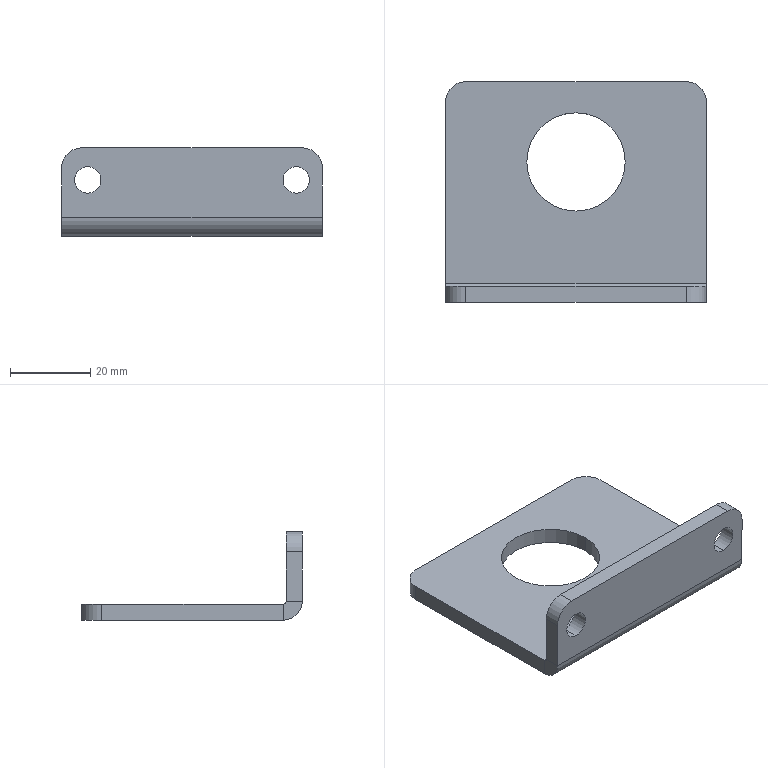Part | SolidWorks | features EdgeFlange 1, Fillet 1, FlatPattern 1, HoleWzd 1, ICE 1, SMBaseFlange 1, SheetMetal 1 | 1 solid | 24 faces | box 65 x 55 x 22 mm | volume 16429 mm3 | cylinder 12 | plane 12 | commonest cylinder face diameters 6.6 x4 10 x4 24.5 x2 1.473 x1 9.473 x1
STEP:
#1=CARTESIAN_POINT('',(-26.,-27.5,6.7));
#2=VERTEX_POINT('',#1);
#3=CARTESIAN_POINT('',(-26.,-27.5,13.3));
#4=VERTEX_POINT('',#3);
#5=CARTESIAN_POINT('',(-26.,-27.5,10.));
#6=DIRECTION('',(0.,1.,0.));
#7=DIRECTION('',(0.,0.,1.));
#8=AXIS2_PLACEMENT_3D('',#5,#6,#7);
#9=CIRCLE('',#8,3.3);
#10=EDGE_CURVE('',#2,#4,#9,.T.);
#11=ORIENTED_EDGE('',*,*,#10,.F.);
#12=CARTESIAN_POINT('',(-26.,-23.5,6.7));
#13=VERTEX_POINT('',#12);
#14=CARTESIAN_POINT('',(-26.,-23.5,6.7));
#15=DIRECTION('',(0.,1.,0.));
#16=VECTOR('',#15,1000.);
#17=LINE('',#14,#16);
#18=EDGE_CURVE('',#2,#13,#17,.T.);
#19=ORIENTED_EDGE('',*,*,#18,.T.);
#20=CARTESIAN_POINT('',(-26.,-23.5,13.3));
#21=VERTEX_POINT('',#20);
#22=CARTESIAN_POINT('',(-26.,-23.5,10.));
#23=DIRECTION('',(0.,1.,0.));
#24=DIRECTION('',(0.,0.,1.));
#25=AXIS2_PLACEMENT_3D('',#22,#23,#24);
#26=CIRCLE('',#25,3.3);
#27=EDGE_CURVE('',#13,#21,#26,.T.);
#28=ORIENTED_EDGE('',*,*,#27,.T.);
#29=CARTESIAN_POINT('',(-26.,-23.5,13.3));
#30=DIRECTION('',(0.,1.,0.));
#31=VECTOR('',#30,1000.);
#32=LINE('',#29,#31);
#33=EDGE_CURVE('',#4,#21,#32,.T.);
#34=ORIENTED_EDGE('',*,*,#33,.F.);
#35=EDGE_LOOP('',(#11,#19,#28,#34));
#36=FACE_OUTER_BOUND('',#35,.T.);
#37=CARTESIAN_POINT('',(-26.,-23.5,10.));
#38=DIRECTION('',(0.,1.,0.));
#39=DIRECTION('',(0.,0.,1.));
#40=AXIS2_PLACEMENT_3D('',#37,#38,#39);
#41=CYLINDRICAL_SURFACE('',#40,3.3);
#42=ADVANCED_FACE('',(#36),#41,.F.);
#43=CARTESIAN_POINT('',(26.,-27.5,6.7));
#44=VERTEX_POINT('',#43);
#45=CARTESIAN_POINT('',(26.,-27.5,13.3));
#46=VERTEX_POINT('',#45);
#47=CARTESIAN_POINT('',(26.,-27.5,10.));
#48=DIRECTION('',(0.,1.,0.));
#49=DIRECTION('',(0.,0.,1.));
#50=AXIS2_PLACEMENT_3D('',#47,#48,#49);
#51=CIRCLE('',#50,3.3);
#52=EDGE_CURVE('',#44,#46,#51,.T.);
#53=ORIENTED_EDGE('',*,*,#52,.F.);
#54=CARTESIAN_POINT('',(26.,-23.5,6.7));
#55=VERTEX_POINT('',#54);
#56=CARTESIAN_POINT('',(26.,-23.5,6.7));
#57=DIRECTION('',(0.,1.,0.));
#58=VECTOR('',#57,1000.);
#59=LINE('',#56,#58);
#60=EDGE_CURVE('',#44,#55,#59,.T.);
#61=ORIENTED_EDGE('',*,*,#60,.T.);
#62=CARTESIAN_POINT('',(26.,-23.5,13.3));
#63=VERTEX_POINT('',#62);
#64=CARTESIAN_POINT('',(26.,-23.5,10.));
#65=DIRECTION('',(0.,1.,0.));
#66=DIRECTION('',(0.,0.,1.));
#67=AXIS2_PLACEMENT_3D('',#64,#65,#66);
#68=CIRCLE('',#67,3.3);
#69=EDGE_CURVE('',#55,#63,#68,.T.);
#70=ORIENTED_EDGE('',*,*,#69,.T.);
#71=CARTESIAN_POINT('',(26.,-23.5,13.3));
#72=DIRECTION('',(0.,1.,0.));
#73=VECTOR('',#72,1000.);
#74=LINE('',#71,#73);
#75=EDGE_CURVE('',#46,#63,#74,.T.);
#76=ORIENTED_EDGE('',*,*,#75,.F.);
#77=EDGE_LOOP('',(#53,#61,#70,#76));
#78=FACE_OUTER_BOUND('',#77,.T.);
#79=CARTESIAN_POINT('',(26.,-23.5,10.));
#80=DIRECTION('',(0.,1.,0.));
#81=DIRECTION('',(0.,0.,1.));
#82=AXIS2_PLACEMENT_3D('',#79,#80,#81);
#83=CYLINDRICAL_SURFACE('',#82,3.3);
#84=ADVANCED_FACE('',(#78),#83,.F.);
#85=CARTESIAN_POINT('',(12.25,7.5,0.));
#86=VERTEX_POINT('',#85);
#87=CARTESIAN_POINT('',(-12.25,7.5,0.));
#88=VERTEX_POINT('',#87);
#89=CARTESIAN_POINT('',(0.,7.5,0.));
#90=DIRECTION('',(0.,0.,-1.));
#91=DIRECTION('',(-1.,0.,0.));
#92=AXIS2_PLACEMENT_3D('',#89,#90,#91);
#93=CIRCLE('',#92,12.25);
#94=EDGE_CURVE('',#86,#88,#93,.T.);
#95=ORIENTED_EDGE('',*,*,#94,.F.);
#96=CARTESIAN_POINT('',(12.25,7.5,-4.));
#97=VERTEX_POINT('',#96);
#98=CARTESIAN_POINT('',(12.25,7.5,18.));
#99=DIRECTION('',(0.,0.,-1.));
#100=VECTOR('',#99,1000.);
#101=LINE('',#98,#100);
#102=EDGE_CURVE('',#86,#97,#101,.T.);
#103=ORIENTED_EDGE('',*,*,#102,.T.);
#104=CARTESIAN_POINT('',(-12.25,7.5,-4.));
#105=VERTEX_POINT('',#104);
#106=CARTESIAN_POINT('',(0.,7.5,-4.));
#107=DIRECTION('',(0.,0.,-1.));
#108=DIRECTION('',(-1.,0.,0.));
#109=AXIS2_PLACEMENT_3D('',#106,#107,#108);
#110=CIRCLE('',#109,12.25);
#111=EDGE_CURVE('',#97,#105,#110,.T.);
#112=ORIENTED_EDGE('',*,*,#111,.T.);
#113=CARTESIAN_POINT('',(-12.25,7.5,18.));
#114=DIRECTION('',(0.,0.,-1.));
#115=VECTOR('',#114,1000.);
#116=LINE('',#113,#115);
#117=EDGE_CURVE('',#88,#105,#116,.T.);
#118=ORIENTED_EDGE('',*,*,#117,.F.);
#119=EDGE_LOOP('',(#95,#103,#112,#118));
#120=FACE_OUTER_BOUND('',#119,.T.);
#121=CARTESIAN_POINT('',(0.,7.5,18.));
#122=DIRECTION('',(0.,0.,-1.));
#123=DIRECTION('',(-1.,0.,0.));
#124=AXIS2_PLACEMENT_3D('',#121,#122,#123);
#125=CYLINDRICAL_SURFACE('',#124,12.25);
#126=ADVANCED_FACE('',(#120),#125,.F.);
#127=CARTESIAN_POINT('',(32.5,-22.763,-4.));
#128=VERTEX_POINT('',#127);
#129=CARTESIAN_POINT('',(32.5,22.5,-4.));
#130=VERTEX_POINT('',#129);
#131=CARTESIAN_POINT('',(32.5,-27.5,-4.));
#132=DIRECTION('',(0.,1.,0.));
#133=VECTOR('',#132,1000.);
#134=LINE('',#131,#133);
#135=EDGE_CURVE('',#128,#130,#134,.T.);
#136=ORIENTED_EDGE('',*,*,#135,.T.);
#137=CARTESIAN_POINT('',(32.5,22.5,0.));
#138=VERTEX_POINT('',#137);
#139=CARTESIAN_POINT('',(32.5,22.5,-4.));
#140=DIRECTION('',(0.,0.,1.));
#141=VECTOR('',#140,1000.);
#142=LINE('',#139,#141);
#143=EDGE_CURVE('',#130,#138,#142,.T.);
#144=ORIENTED_EDGE('',*,*,#143,.T.);
#145=CARTESIAN_POINT('',(32.5,-22.763,0.));
#146=VERTEX_POINT('',#145);
#147=CARTESIAN_POINT('',(32.5,-27.5,0.));
#148=DIRECTION('',(0.,1.,0.));
#149=VECTOR('',#148,1000.);
#150=LINE('',#147,#149);
#151=EDGE_CURVE('',#146,#138,#150,.T.);
#152=ORIENTED_EDGE('',*,*,#151,.F.);
#153=CARTESIAN_POINT('',(32.5,-22.763,0.));
#154=DIRECTION('',(0.,0.,-1.));
#155=VECTOR('',#154,1000.);
#156=LINE('',#153,#155);
#157=EDGE_CURVE('',#146,#128,#156,.T.);
#158=ORIENTED_EDGE('',*,*,#157,.T.);
#159=EDGE_LOOP('',(#136,#144,#152,#158));
#160=FACE_OUTER_BOUND('',#159,.T.);
#161=CARTESIAN_POINT('',(32.5,-27.5,-4.));
#162=DIRECTION('',(1.,0.,0.));
#163=DIRECTION('',(0.,0.,-1.));
#164=AXIS2_PLACEMENT_3D('',#161,#162,#163);
#165=PLANE('',#164);
#166=ADVANCED_FACE('',(#160),#165,.T.);
#167=CARTESIAN_POINT('',(0.,7.5,-4.));
#168=DIRECTION('',(0.,0.,-1.));
#169=DIRECTION('',(-1.,0.,0.));
#170=AXIS2_PLACEMENT_3D('',#167,#168,#169);
#171=CIRCLE('',#170,12.25);
#172=EDGE_CURVE('',#105,#97,#171,.T.);
#173=ORIENTED_EDGE('',*,*,#172,.F.);
#174=ORIENTED_EDGE('',*,*,#111,.F.);
#175=EDGE_LOOP('',(#173,#174));
#176=FACE_BOUND('',#175,.T.);
#177=CARTESIAN_POINT('',(27.5,27.5,-4.));
#178=VERTEX_POINT('',#177);
#179=CARTESIAN_POINT('',(-27.5,27.5,-4.));
#180=VERTEX_POINT('',#179);
#181=CARTESIAN_POINT('',(-32.5,27.5,-4.));
#182=DIRECTION('',(-1.,0.,0.));
#183=VECTOR('',#182,1000.);
#184=LINE('',#181,#183);
#185=EDGE_CURVE('',#178,#180,#184,.T.);
#186=ORIENTED_EDGE('',*,*,#185,.F.);
#187=CARTESIAN_POINT('',(27.5,22.5,-4.));
#188=DIRECTION('',(0.,0.,-1.));
#189=DIRECTION('',(-1.,0.,0.));
#190=AXIS2_PLACEMENT_3D('',#187,#188,#189);
#191=CIRCLE('',#190,5.);
#192=EDGE_CURVE('',#178,#130,#191,.T.);
#193=ORIENTED_EDGE('',*,*,#192,.T.);
#194=ORIENTED_EDGE('',*,*,#135,.F.);
#195=CARTESIAN_POINT('',(-32.5,-22.763,-4.));
#196=VERTEX_POINT('',#195);
#197=CARTESIAN_POINT('',(32.5,-22.763,-4.));
#198=DIRECTION('',(-1.,0.,0.));
#199=VECTOR('',#198,1000.);
#200=LINE('',#197,#199);
#201=EDGE_CURVE('',#128,#196,#200,.T.);
#202=ORIENTED_EDGE('',*,*,#201,.T.);
#203=CARTESIAN_POINT('',(-32.5,22.5,-4.));
#204=VERTEX_POINT('',#203);
#205=CARTESIAN_POINT('',(-32.5,-27.5,-4.));
#206=DIRECTION('',(0.,-1.,0.));
#207=VECTOR('',#206,1000.);
#208=LINE('',#205,#207);
#209=EDGE_CURVE('',#204,#196,#208,.T.);
#210=ORIENTED_EDGE('',*,*,#209,.F.);
#211=CARTESIAN_POINT('',(-27.5,22.5,-4.));
#212=DIRECTION('',(0.,0.,-1.));
#213=DIRECTION('',(-1.,0.,0.));
#214=AXIS2_PLACEMENT_3D('',#211,#212,#213);
#215=CIRCLE('',#214,5.);
#216=EDGE_CURVE('',#204,#180,#215,.T.);
#217=ORIENTED_EDGE('',*,*,#216,.T.);
#218=EDGE_LOOP('',(#186,#193,#194,#202,#210,#217));
#219=FACE_OUTER_BOUND('',#218,.T.);
#220=CARTESIAN_POINT('',(0.,0.,-4.));
#221=DIRECTION('',(0.,0.,-1.));
#222=DIRECTION('',(-1.,0.,0.));
#223=AXIS2_PLACEMENT_3D('',#220,#221,#222);
#224=PLANE('',#223);
#225=ADVANCED_FACE('',(#176,#219),#224,.T.);
#226=CARTESIAN_POINT('',(0.,7.5,0.));
#227=DIRECTION('',(0.,0.,-1.));
#228=DIRECTION('',(-1.,0.,0.));
#229=AXIS2_PLACEMENT_3D('',#226,#227,#228);
#230=CIRCLE('',#229,12.25);
#231=EDGE_CURVE('',#88,#86,#230,.T.);
#232=ORIENTED_EDGE('',*,*,#231,.T.);
#233=ORIENTED_EDGE('',*,*,#94,.T.);
#234=EDGE_LOOP('',(#232,#233));
#235=FACE_BOUND('',#234,.T.);
#236=ORIENTED_EDGE('',*,*,#151,.T.);
#237=CARTESIAN_POINT('',(27.5,27.5,0.));
#238=VERTEX_POINT('',#237);
#239=CARTESIAN_POINT('',(27.5,22.5,0.));
#240=DIRECTION('',(0.,0.,1.));
#241=DIRECTION('',(-1.,0.,0.));
#242=AXIS2_PLACEMENT_3D('',#239,#240,#241);
#243=CIRCLE('',#242,5.);
#244=EDGE_CURVE('',#138,#238,#243,.T.);
#245=ORIENTED_EDGE('',*,*,#244,.T.);
#246=CARTESIAN_POINT('',(-27.5,27.5,0.));
#247=VERTEX_POINT('',#246);
#248=CARTESIAN_POINT('',(-32.5,27.5,0.));
#249=DIRECTION('',(-1.,0.,0.));
#250=VECTOR('',#249,1000.);
#251=LINE('',#248,#250);
#252=EDGE_CURVE('',#238,#247,#251,.T.);
#253=ORIENTED_EDGE('',*,*,#252,.T.);
#254=CARTESIAN_POINT('',(-32.5,22.5,0.));
#255=VERTEX_POINT('',#254);
#256=CARTESIAN_POINT('',(-27.5,22.5,0.));
#257=DIRECTION('',(0.,0.,1.));
#258=DIRECTION('',(-1.,0.,0.));
#259=AXIS2_PLACEMENT_3D('',#256,#257,#258);
#260=CIRCLE('',#259,5.);
#261=EDGE_CURVE('',#247,#255,#260,.T.);
#262=ORIENTED_EDGE('',*,*,#261,.T.);
#263=CARTESIAN_POINT('',(-32.5,-22.763,0.));
#264=VERTEX_POINT('',#263);
#265=CARTESIAN_POINT('',(-32.5,-27.5,0.));
#266=DIRECTION('',(0.,-1.,0.));
#267=VECTOR('',#266,1000.);
#268=LINE('',#265,#267);
#269=EDGE_CURVE('',#255,#264,#268,.T.);
#270=ORIENTED_EDGE('',*,*,#269,.T.);
#271=CARTESIAN_POINT('',(32.5,-22.763,0.));
#272=DIRECTION('',(-1.,0.,0.));
#273=VECTOR('',#272,1000.);
#274=LINE('',#271,#273);
#275=EDGE_CURVE('',#146,#264,#274,.T.);
#276=ORIENTED_EDGE('',*,*,#275,.F.);
#277=EDGE_LOOP('',(#236,#245,#253,#262,#270,#276));
#278=FACE_OUTER_BOUND('',#277,.T.);
#279=CARTESIAN_POINT('',(0.,0.,0.));
#280=DIRECTION('',(0.,0.,-1.));
#281=DIRECTION('',(-1.,0.,0.));
#282=AXIS2_PLACEMENT_3D('',#279,#280,#281);
#283=PLANE('',#282);
#284=ADVANCED_FACE('',(#235,#278),#283,.F.);
#285=ORIENTED_EDGE('',*,*,#269,.F.);
#286=CARTESIAN_POINT('',(-32.5,22.5,-4.));
#287=DIRECTION('',(0.,0.,-1.));
#288=VECTOR('',#287,1000.);
#289=LINE('',#286,#288);
#290=EDGE_CURVE('',#255,#204,#289,.T.);
#291=ORIENTED_EDGE('',*,*,#290,.T.);
#292=ORIENTED_EDGE('',*,*,#209,.T.);
#293=CARTESIAN_POINT('',(-32.5,-22.763,0.));
#294=DIRECTION('',(0.,0.,-1.));
#295=VECTOR('',#294,1000.);
#296=LINE('',#293,#295);
#297=EDGE_CURVE('',#264,#196,#296,.T.);
#298=ORIENTED_EDGE('',*,*,#297,.F.);
#299=EDGE_LOOP('',(#285,#291,#292,#298));
#300=FACE_OUTER_BOUND('',#299,.T.);
#301=CARTESIAN_POINT('',(-32.5,-27.5,-4.));
#302=DIRECTION('',(-1.,0.,0.));
#303=DIRECTION('',(0.,0.,1.));
#304=AXIS2_PLACEMENT_3D('',#301,#302,#303);
#305=PLANE('',#304);
#306=ADVANCED_FACE('',(#300),#305,.T.);
#307=ORIENTED_EDGE('',*,*,#252,.F.);
#308=CARTESIAN_POINT('',(27.5,27.5,-4.));
#309=DIRECTION('',(0.,0.,-1.));
#310=VECTOR('',#309,1000.);
#311=LINE('',#308,#310);
#312=EDGE_CURVE('',#238,#178,#311,.T.);
#313=ORIENTED_EDGE('',*,*,#312,.T.);
#314=ORIENTED_EDGE('',*,*,#185,.T.);
#315=CARTESIAN_POINT('',(-27.5,27.5,-4.));
#316=DIRECTION('',(0.,0.,1.));
#317=VECTOR('',#316,1000.);
#318=LINE('',#315,#317);
#319=EDGE_CURVE('',#180,#247,#318,.T.);
#320=ORIENTED_EDGE('',*,*,#319,.T.);
#321=EDGE_LOOP('',(#307,#313,#314,#320));
#322=FACE_OUTER_BOUND('',#321,.T.);
#323=CARTESIAN_POINT('',(-32.5,27.5,-4.));
#324=DIRECTION('',(0.,1.,0.));
#325=DIRECTION('',(0.,0.,1.));
#326=AXIS2_PLACEMENT_3D('',#323,#324,#325);
#327=PLANE('',#326);
#328=ADVANCED_FACE('',(#322),#327,.T.);
#329=CARTESIAN_POINT('',(-32.5,-23.5,0.7366));
#330=VERTEX_POINT('',#329);
#331=CARTESIAN_POINT('',(-32.5,-27.5,0.7366));
#332=VERTEX_POINT('',#331);
#333=CARTESIAN_POINT('',(-32.5,-27.5,0.7366));
#334=DIRECTION('',(0.,-1.,0.));
#335=VECTOR('',#334,1000.);
#336=LINE('',#333,#335);
#337=EDGE_CURVE('',#330,#332,#336,.T.);
#338=ORIENTED_EDGE('',*,*,#337,.F.);
#339=CARTESIAN_POINT('',(-32.5,-22.763,0.7366));
#340=DIRECTION('',(-1.,0.,0.));
#341=DIRECTION('',(0.,0.,-1.));
#342=AXIS2_PLACEMENT_3D('',#339,#340,#341);
#343=CIRCLE('',#342,0.7366);
#344=EDGE_CURVE('',#264,#330,#343,.T.);
#345=ORIENTED_EDGE('',*,*,#344,.F.);
#346=ORIENTED_EDGE('',*,*,#297,.T.);
#347=CARTESIAN_POINT('',(-32.5,-22.763,0.7366));
#348=DIRECTION('',(-1.,0.,0.));
#349=DIRECTION('',(0.,0.,-1.));
#350=AXIS2_PLACEMENT_3D('',#347,#348,#349);
#351=CIRCLE('',#350,4.737);
#352=EDGE_CURVE('',#196,#332,#351,.T.);
#353=ORIENTED_EDGE('',*,*,#352,.T.);
#354=EDGE_LOOP('',(#338,#345,#346,#353));
#355=FACE_OUTER_BOUND('',#354,.T.);
#356=CARTESIAN_POINT('',(-32.5,-22.763,0.7366));
#357=DIRECTION('',(-1.,0.,0.));
#358=DIRECTION('',(0.,0.,1.));
#359=AXIS2_PLACEMENT_3D('',#356,#357,#358);
#360=PLANE('',#359);
#361=ADVANCED_FACE('',(#355),#360,.T.);
#362=CARTESIAN_POINT('',(32.5,-23.5,0.7366));
#363=VERTEX_POINT('',#362);
#364=CARTESIAN_POINT('',(32.5,-22.763,0.7366));
#365=DIRECTION('',(1.,0.,0.));
#366=DIRECTION('',(0.,0.,-1.));
#367=AXIS2_PLACEMENT_3D('',#364,#365,#366);
#368=CIRCLE('',#367,0.7366);
#369=EDGE_CURVE('',#363,#146,#368,.T.);
#370=ORIENTED_EDGE('',*,*,#369,.F.);
#371=CARTESIAN_POINT('',(32.5,-27.5,0.7366));
#372=VERTEX_POINT('',#371);
#373=CARTESIAN_POINT('',(32.5,-23.5,0.7366));
#374=DIRECTION('',(0.,-1.,0.));
#375=VECTOR('',#374,1000.);
#376=LINE('',#373,#375);
#377=EDGE_CURVE('',#363,#372,#376,.T.);
#378=ORIENTED_EDGE('',*,*,#377,.T.);
#379=CARTESIAN_POINT('',(32.5,-22.763,0.7366));
#380=DIRECTION('',(1.,0.,0.));
#381=DIRECTION('',(0.,0.,-1.));
#382=AXIS2_PLACEMENT_3D('',#379,#380,#381);
#383=CIRCLE('',#382,4.737);
#384=EDGE_CURVE('',#372,#128,#383,.T.);
#385=ORIENTED_EDGE('',*,*,#384,.T.);
#386=ORIENTED_EDGE('',*,*,#157,.F.);
#387=EDGE_LOOP('',(#370,#378,#385,#386));
#388=FACE_OUTER_BOUND('',#387,.T.);
#389=CARTESIAN_POINT('',(32.5,-22.763,0.7366));
#390=DIRECTION('',(-1.,0.,0.));
#391=DIRECTION('',(0.,0.,1.));
#392=AXIS2_PLACEMENT_3D('',#389,#390,#391);
#393=PLANE('',#392);
#394=ADVANCED_FACE('',(#388),#393,.F.);
#395=ORIENTED_EDGE('',*,*,#201,.F.);
#396=ORIENTED_EDGE('',*,*,#384,.F.);
#397=CARTESIAN_POINT('',(-32.5,-27.5,0.7366));
#398=DIRECTION('',(-1.,0.,0.));
#399=VECTOR('',#398,1000.);
#400=LINE('',#397,#399);
#401=EDGE_CURVE('',#372,#332,#400,.T.);
#402=ORIENTED_EDGE('',*,*,#401,.T.);
#403=ORIENTED_EDGE('',*,*,#352,.F.);
#404=EDGE_LOOP('',(#395,#396,#402,#403));
#405=FACE_OUTER_BOUND('',#404,.T.);
#406=CARTESIAN_POINT('',(32.5,-22.763,0.7366));
#407=DIRECTION('',(1.,0.,0.));
#408=DIRECTION('',(0.,-1.,0.));
#409=AXIS2_PLACEMENT_3D('',#406,#407,#408);
#410=CYLINDRICAL_SURFACE('',#409,4.737);
#411=ADVANCED_FACE('',(#405),#410,.T.);
#412=ORIENTED_EDGE('',*,*,#275,.T.);
#413=ORIENTED_EDGE('',*,*,#344,.T.);
#414=CARTESIAN_POINT('',(-32.5,-23.5,0.7366));
#415=DIRECTION('',(1.,0.,0.));
#416=VECTOR('',#415,1000.);
#417=LINE('',#414,#416);
#418=EDGE_CURVE('',#330,#363,#417,.T.);
#419=ORIENTED_EDGE('',*,*,#418,.T.);
#420=ORIENTED_EDGE('',*,*,#369,.T.);
#421=EDGE_LOOP('',(#412,#413,#419,#420));
#422=FACE_OUTER_BOUND('',#421,.T.);
#423=CARTESIAN_POINT('',(32.5,-22.763,0.7366));
#424=DIRECTION('',(1.,0.,0.));
#425=DIRECTION('',(0.,-1.,0.));
#426=AXIS2_PLACEMENT_3D('',#423,#424,#425);
#427=CYLINDRICAL_SURFACE('',#426,0.7366);
#428=ADVANCED_FACE('',(#422),#427,.F.);
#429=CARTESIAN_POINT('',(-32.5,-27.5,13.));
#430=VERTEX_POINT('',#429);
#431=CARTESIAN_POINT('',(-32.5,-27.5,0.));
#432=DIRECTION('',(0.,0.,-1.));
#433=VECTOR('',#432,1000.);
#434=LINE('',#431,#433);
#435=EDGE_CURVE('',#430,#332,#434,.T.);
#436=ORIENTED_EDGE('',*,*,#435,.F.);
#437=CARTESIAN_POINT('',(-32.5,-23.5,13.));
#438=VERTEX_POINT('',#437);
#439=CARTESIAN_POINT('',(-32.5,-27.5,13.));
#440=DIRECTION('',(0.,1.,0.));
#441=VECTOR('',#440,1000.);
#442=LINE('',#439,#441);
#443=EDGE_CURVE('',#430,#438,#442,.T.);
#444=ORIENTED_EDGE('',*,*,#443,.T.);
#445=CARTESIAN_POINT('',(-32.5,-23.5,0.));
#446=DIRECTION('',(0.,0.,-1.));
#447=VECTOR('',#446,1000.);
#448=LINE('',#445,#447);
#449=EDGE_CURVE('',#438,#330,#448,.T.);
#450=ORIENTED_EDGE('',*,*,#449,.T.);
#451=ORIENTED_EDGE('',*,*,#337,.T.);
#452=EDGE_LOOP('',(#436,#444,#450,#451));
#453=FACE_OUTER_BOUND('',#452,.T.);
#454=CARTESIAN_POINT('',(-32.5,-27.5,0.));
#455=DIRECTION('',(1.,0.,0.));
#456=DIRECTION('',(0.,0.,-1.));
#457=AXIS2_PLACEMENT_3D('',#454,#455,#456);
#458=PLANE('',#457);
#459=ADVANCED_FACE('',(#453),#458,.F.);
#460=CARTESIAN_POINT('',(32.5,-23.5,13.));
#461=VERTEX_POINT('',#460);
#462=CARTESIAN_POINT('',(32.5,-23.5,18.));
#463=DIRECTION('',(0.,0.,1.));
#464=VECTOR('',#463,1000.);
#465=LINE('',#462,#464);
#466=EDGE_CURVE('',#363,#461,#465,.T.);
#467=ORIENTED_EDGE('',*,*,#466,.T.);
#468=CARTESIAN_POINT('',(32.5,-27.5,13.));
#469=VERTEX_POINT('',#468);
#470=CARTESIAN_POINT('',(32.5,-27.5,13.));
#471=DIRECTION('',(0.,-1.,0.));
#472=VECTOR('',#471,1000.);
#473=LINE('',#470,#472);
#474=EDGE_CURVE('',#461,#469,#473,.T.);
#475=ORIENTED_EDGE('',*,*,#474,.T.);
#476=CARTESIAN_POINT('',(32.5,-27.5,0.));
#477=DIRECTION('',(0.,0.,1.));
#478=VECTOR('',#477,1000.);
#479=LINE('',#476,#478);
#480=EDGE_CURVE('',#372,#469,#479,.T.);
#481=ORIENTED_EDGE('',*,*,#480,.F.);
#482=ORIENTED_EDGE('',*,*,#377,.F.);
#483=EDGE_LOOP('',(#467,#475,#481,#482));
#484=FACE_OUTER_BOUND('',#483,.T.);
#485=CARTESIAN_POINT('',(32.5,-27.5,18.));
#486=DIRECTION('',(-1.,0.,0.));
#487=DIRECTION('',(0.,0.,1.));
#488=AXIS2_PLACEMENT_3D('',#485,#486,#487);
#489=PLANE('',#488);
#490=ADVANCED_FACE('',(#484),#489,.F.);
#491=CARTESIAN_POINT('',(-26.,-27.5,10.));
#492=DIRECTION('',(0.,1.,0.));
#493=DIRECTION('',(0.,0.,1.));
#494=AXIS2_PLACEMENT_3D('',#491,#492,#493);
#495=CIRCLE('',#494,3.3);
#496=EDGE_CURVE('',#4,#2,#495,.T.);
#497=ORIENTED_EDGE('',*,*,#496,.T.);
#498=ORIENTED_EDGE('',*,*,#10,.T.);
#499=EDGE_LOOP('',(#497,#498));
#500=FACE_BOUND('',#499,.T.);
#501=CARTESIAN_POINT('',(26.,-27.5,10.));
#502=DIRECTION('',(0.,1.,0.));
#503=DIRECTION('',(0.,0.,1.));
#504=AXIS2_PLACEMENT_3D('',#501,#502,#503);
#505=CIRCLE('',#504,3.3);
#506=EDGE_CURVE('',#46,#44,#505,.T.);
#507=ORIENTED_EDGE('',*,*,#506,.T.);
#508=ORIENTED_EDGE('',*,*,#52,.T.);
#509=EDGE_LOOP('',(#507,#508));
#510=FACE_BOUND('',#509,.T.);
#511=ORIENTED_EDGE('',*,*,#480,.T.);
#512=CARTESIAN_POINT('',(27.5,-27.5,18.));
#513=VERTEX_POINT('',#512);
#514=CARTESIAN_POINT('',(27.5,-27.5,13.));
#515=DIRECTION('',(0.,-1.,0.));
#516=DIRECTION('',(0.,0.,1.));
#517=AXIS2_PLACEMENT_3D('',#514,#515,#516);
#518=CIRCLE('',#517,5.);
#519=EDGE_CURVE('',#469,#513,#518,.T.);
#520=ORIENTED_EDGE('',*,*,#519,.T.);
#521=CARTESIAN_POINT('',(-27.5,-27.5,18.));
#522=VERTEX_POINT('',#521);
#523=CARTESIAN_POINT('',(0.,-27.5,18.));
#524=DIRECTION('',(-1.,0.,0.));
#525=VECTOR('',#524,1000.);
#526=LINE('',#523,#525);
#527=EDGE_CURVE('',#513,#522,#526,.T.);
#528=ORIENTED_EDGE('',*,*,#527,.T.);
#529=CARTESIAN_POINT('',(-27.5,-27.5,13.));
#530=DIRECTION('',(0.,-1.,0.));
#531=DIRECTION('',(0.,0.,1.));
#532=AXIS2_PLACEMENT_3D('',#529,#530,#531);
#533=CIRCLE('',#532,5.);
#534=EDGE_CURVE('',#522,#430,#533,.T.);
#535=ORIENTED_EDGE('',*,*,#534,.T.);
#536=ORIENTED_EDGE('',*,*,#435,.T.);
#537=ORIENTED_EDGE('',*,*,#401,.F.);
#538=EDGE_LOOP('',(#511,#520,#528,#535,#536,#537));
#539=FACE_OUTER_BOUND('',#538,.T.);
#540=CARTESIAN_POINT('',(0.,-27.5,0.));
#541=DIRECTION('',(0.,1.,0.));
#542=DIRECTION('',(0.,0.,1.));
#543=AXIS2_PLACEMENT_3D('',#540,#541,#542);
#544=PLANE('',#543);
#545=ADVANCED_FACE('',(#500,#510,#539),#544,.F.);
#546=CARTESIAN_POINT('',(-26.,-23.5,10.));
#547=DIRECTION('',(0.,1.,0.));
#548=DIRECTION('',(0.,0.,1.));
#549=AXIS2_PLACEMENT_3D('',#546,#547,#548);
#550=CIRCLE('',#549,3.3);
#551=EDGE_CURVE('',#21,#13,#550,.T.);
#552=ORIENTED_EDGE('',*,*,#551,.F.);
#553=ORIENTED_EDGE('',*,*,#27,.F.);
#554=EDGE_LOOP('',(#552,#553));
#555=FACE_BOUND('',#554,.T.);
#556=CARTESIAN_POINT('',(26.,-23.5,10.));
#557=DIRECTION('',(0.,1.,0.));
#558=DIRECTION('',(0.,0.,1.));
#559=AXIS2_PLACEMENT_3D('',#556,#557,#558);
#560=CIRCLE('',#559,3.3);
#561=EDGE_CURVE('',#63,#55,#560,.T.);
#562=ORIENTED_EDGE('',*,*,#561,.F.);
#563=ORIENTED_EDGE('',*,*,#69,.F.);
#564=EDGE_LOOP('',(#562,#563));
#565=FACE_BOUND('',#564,.T.);
#566=CARTESIAN_POINT('',(27.5,-23.5,18.));
#567=VERTEX_POINT('',#566);
#568=CARTESIAN_POINT('',(-27.5,-23.5,18.));
#569=VERTEX_POINT('',#568);
#570=CARTESIAN_POINT('',(-32.5,-23.5,18.));
#571=DIRECTION('',(-1.,0.,0.));
#572=VECTOR('',#571,1000.);
#573=LINE('',#570,#572);
#574=EDGE_CURVE('',#567,#569,#573,.T.);
#575=ORIENTED_EDGE('',*,*,#574,.F.);
#576=CARTESIAN_POINT('',(27.5,-23.5,13.));
#577=DIRECTION('',(0.,1.,0.));
#578=DIRECTION('',(0.,0.,1.));
#579=AXIS2_PLACEMENT_3D('',#576,#577,#578);
#580=CIRCLE('',#579,5.);
#581=EDGE_CURVE('',#567,#461,#580,.T.);
#582=ORIENTED_EDGE('',*,*,#581,.T.);
#583=ORIENTED_EDGE('',*,*,#466,.F.);
#584=ORIENTED_EDGE('',*,*,#418,.F.);
#585=ORIENTED_EDGE('',*,*,#449,.F.);
#586=CARTESIAN_POINT('',(-27.5,-23.5,13.));
#587=DIRECTION('',(0.,1.,0.));
#588=DIRECTION('',(0.,0.,1.));
#589=AXIS2_PLACEMENT_3D('',#586,#587,#588);
#590=CIRCLE('',#589,5.);
#591=EDGE_CURVE('',#438,#569,#590,.T.);
#592=ORIENTED_EDGE('',*,*,#591,.T.);
#593=EDGE_LOOP('',(#575,#582,#583,#584,#585,#592));
#594=FACE_OUTER_BOUND('',#593,.T.);
#595=CARTESIAN_POINT('',(0.,-23.5,0.));
#596=DIRECTION('',(0.,1.,0.));
#597=DIRECTION('',(0.,0.,1.));
#598=AXIS2_PLACEMENT_3D('',#595,#596,#597);
#599=PLANE('',#598);
#600=ADVANCED_FACE('',(#555,#565,#594),#599,.T.);
#601=ORIENTED_EDGE('',*,*,#527,.F.);
#602=CARTESIAN_POINT('',(27.5,-27.5,18.));
#603=DIRECTION('',(0.,1.,0.));
#604=VECTOR('',#603,1000.);
#605=LINE('',#602,#604);
#606=EDGE_CURVE('',#513,#567,#605,.T.);
#607=ORIENTED_EDGE('',*,*,#606,.T.);
#608=ORIENTED_EDGE('',*,*,#574,.T.);
#609=CARTESIAN_POINT('',(-27.5,-27.5,18.));
#610=DIRECTION('',(0.,-1.,0.));
#611=VECTOR('',#610,1000.);
#612=LINE('',#609,#611);
#613=EDGE_CURVE('',#569,#522,#612,.T.);
#614=ORIENTED_EDGE('',*,*,#613,.T.);
#615=EDGE_LOOP('',(#601,#607,#608,#614));
#616=FACE_OUTER_BOUND('',#615,.T.);
#617=CARTESIAN_POINT('',(-32.5,-27.5,18.));
#618=DIRECTION('',(0.,0.,-1.));
#619=DIRECTION('',(0.,1.,0.));
#620=AXIS2_PLACEMENT_3D('',#617,#618,#619);
#621=PLANE('',#620);
#622=ADVANCED_FACE('',(#616),#621,.F.);
#623=ORIENTED_EDGE('',*,*,#102,.F.);
#624=ORIENTED_EDGE('',*,*,#231,.F.);
#625=ORIENTED_EDGE('',*,*,#117,.T.);
#626=ORIENTED_EDGE('',*,*,#172,.T.);
#627=EDGE_LOOP('',(#623,#624,#625,#626));
#628=FACE_OUTER_BOUND('',#627,.T.);
#629=CARTESIAN_POINT('',(0.,7.5,18.));
#630=DIRECTION('',(0.,0.,-1.));
#631=DIRECTION('',(-1.,0.,0.));
#632=AXIS2_PLACEMENT_3D('',#629,#630,#631);
#633=CYLINDRICAL_SURFACE('',#632,12.25);
#634=ADVANCED_FACE('',(#628),#633,.F.);
#635=ORIENTED_EDGE('',*,*,#60,.F.);
#636=ORIENTED_EDGE('',*,*,#506,.F.);
#637=ORIENTED_EDGE('',*,*,#75,.T.);
#638=ORIENTED_EDGE('',*,*,#561,.T.);
#639=EDGE_LOOP('',(#635,#636,#637,#638));
#640=FACE_OUTER_BOUND('',#639,.T.);
#641=CARTESIAN_POINT('',(26.,-23.5,10.));
#642=DIRECTION('',(0.,1.,0.));
#643=DIRECTION('',(0.,0.,1.));
#644=AXIS2_PLACEMENT_3D('',#641,#642,#643);
#645=CYLINDRICAL_SURFACE('',#644,3.3);
#646=ADVANCED_FACE('',(#640),#645,.F.);
#647=ORIENTED_EDGE('',*,*,#18,.F.);
#648=ORIENTED_EDGE('',*,*,#496,.F.);
#649=ORIENTED_EDGE('',*,*,#33,.T.);
#650=ORIENTED_EDGE('',*,*,#551,.T.);
#651=EDGE_LOOP('',(#647,#648,#649,#650));
#652=FACE_OUTER_BOUND('',#651,.T.);
#653=CARTESIAN_POINT('',(-26.,-23.5,10.));
#654=DIRECTION('',(0.,1.,0.));
#655=DIRECTION('',(0.,0.,1.));
#656=AXIS2_PLACEMENT_3D('',#653,#654,#655);
#657=CYLINDRICAL_SURFACE('',#656,3.3);
#658=ADVANCED_FACE('',(#652),#657,.F.);
#659=ORIENTED_EDGE('',*,*,#192,.F.);
#660=ORIENTED_EDGE('',*,*,#312,.F.);
#661=ORIENTED_EDGE('',*,*,#244,.F.);
#662=ORIENTED_EDGE('',*,*,#143,.F.);
#663=EDGE_LOOP('',(#659,#660,#661,#662));
#664=FACE_OUTER_BOUND('',#663,.T.);
#665=CARTESIAN_POINT('',(27.5,22.5,-4.));
#666=DIRECTION('',(0.,0.,1.));
#667=DIRECTION('',(1.,0.,0.));
#668=AXIS2_PLACEMENT_3D('',#665,#666,#667);
#669=CYLINDRICAL_SURFACE('',#668,5.);
#670=ADVANCED_FACE('',(#664),#669,.T.);
#671=ORIENTED_EDGE('',*,*,#216,.F.);
#672=ORIENTED_EDGE('',*,*,#290,.F.);
#673=ORIENTED_EDGE('',*,*,#261,.F.);
#674=ORIENTED_EDGE('',*,*,#319,.F.);
#675=EDGE_LOOP('',(#671,#672,#673,#674));
#676=FACE_OUTER_BOUND('',#675,.T.);
#677=CARTESIAN_POINT('',(-27.5,22.5,-4.));
#678=DIRECTION('',(0.,0.,1.));
#679=DIRECTION('',(1.,0.,0.));
#680=AXIS2_PLACEMENT_3D('',#677,#678,#679);
#681=CYLINDRICAL_SURFACE('',#680,5.);
#682=ADVANCED_FACE('',(#676),#681,.T.);
#683=ORIENTED_EDGE('',*,*,#519,.F.);
#684=ORIENTED_EDGE('',*,*,#474,.F.);
#685=ORIENTED_EDGE('',*,*,#581,.F.);
#686=ORIENTED_EDGE('',*,*,#606,.F.);
#687=EDGE_LOOP('',(#683,#684,#685,#686));
#688=FACE_OUTER_BOUND('',#687,.T.);
#689=CARTESIAN_POINT('',(27.5,-27.5,13.));
#690=DIRECTION('',(0.,1.,0.));
#691=DIRECTION('',(0.,0.,1.));
#692=AXIS2_PLACEMENT_3D('',#689,#690,#691);
#693=CYLINDRICAL_SURFACE('',#692,5.);
#694=ADVANCED_FACE('',(#688),#693,.T.);
#695=ORIENTED_EDGE('',*,*,#534,.F.);
#696=ORIENTED_EDGE('',*,*,#613,.F.);
#697=ORIENTED_EDGE('',*,*,#591,.F.);
#698=ORIENTED_EDGE('',*,*,#443,.F.);
#699=EDGE_LOOP('',(#695,#696,#697,#698));
#700=FACE_OUTER_BOUND('',#699,.T.);
#701=CARTESIAN_POINT('',(-27.5,-27.5,13.));
#702=DIRECTION('',(0.,1.,0.));
#703=DIRECTION('',(0.,0.,1.));
#704=AXIS2_PLACEMENT_3D('',#701,#702,#703);
#705=CYLINDRICAL_SURFACE('',#704,5.);
#706=ADVANCED_FACE('',(#700),#705,.T.);
#707=CLOSED_SHELL('',(#42,#84,#126,#166,#225,#284,#306,#328,#361,#394,#411,#428,#459,#490,#545,#600,#622,#634,#646,#658,#670,#682,#694,#706));
#708=MANIFOLD_SOLID_BREP('',#707);
#709=CARTESIAN_POINT('',(0.,0.,0.));
#710=DIRECTION('',(0.,0.,1.));
#711=DIRECTION('',(1.,0.,0.));
#712=AXIS2_PLACEMENT_3D('',#709,#710,#711);
#713=(LENGTH_UNIT()NAMED_UNIT(*)SI_UNIT(.MILLI.,.METRE.));
#714=UNCERTAINTY_MEASURE_WITH_UNIT(LENGTH_MEASURE(0.00001),#713,'','');
#715=(NAMED_UNIT(*)PLANE_ANGLE_UNIT()SI_UNIT($,.RADIAN.));
#716=(NAMED_UNIT(*)SI_UNIT($,.STERADIAN.)SOLID_ANGLE_UNIT());
#717=(GEOMETRIC_REPRESENTATION_CONTEXT(3)GLOBAL_UNCERTAINTY_ASSIGNED_CONTEXT((#714))GLOBAL_UNIT_ASSIGNED_CONTEXT((#713,#715,#716))REPRESENTATION_CONTEXT('',''));
#718=ADVANCED_BREP_SHAPE_REPRESENTATION('',(#708,#712),#717);